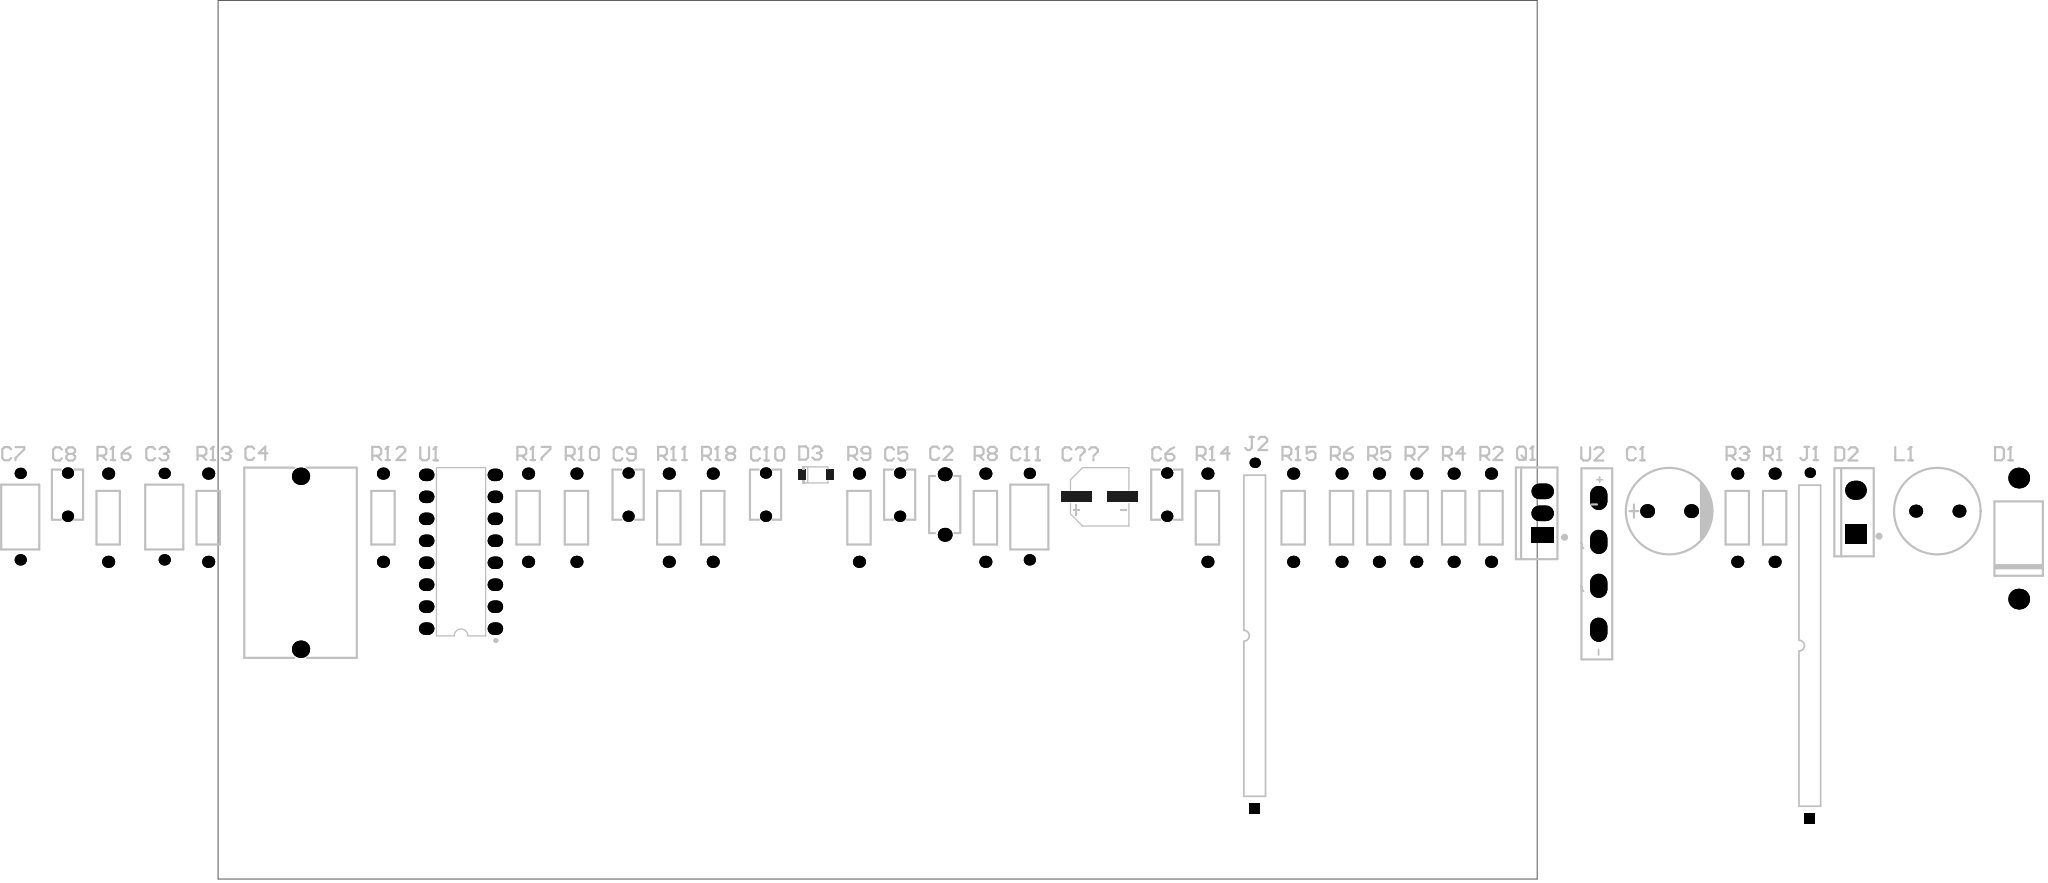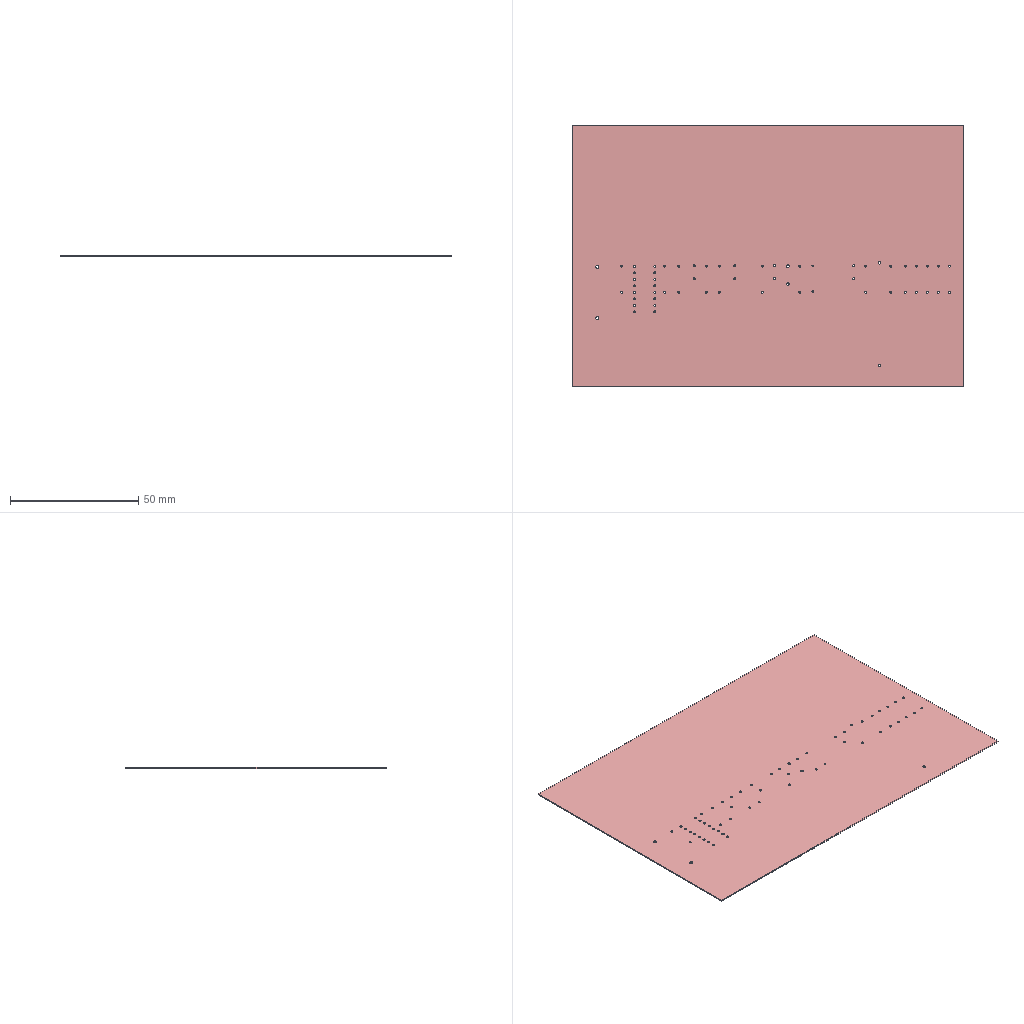Circuit board layout | Altium Designer | box 152.4 x 101.6 x 0.4 mm
Part placement:
Designator,Comment,Layer,Footprint,Center-X(mm),Center-Y(mm),Rotation
U2,GBU8K,TopLayer,GBU_4P-L22.0-W3.5-P5.08-GBU4K,184.912,61.849,90
U1,UC3854N,TopLayer,PDIP-16_L19.3-W6.4-P2.54-LS7.94-BL,53.467,63.246,90
R18,MF1/4W-100K±1%-OT26,TopLayer,RES-TH_BD2.7-L6.2-P10.20-D0.4,82.55,67.183,90
R17,MF1/4W-100K±1%-OT26,TopLayer,RES-TH_BD2.7-L6.2-P10.20-D0.4,61.214,67.183,90
R16,MF1/4W-100K±1%-OT26,TopLayer,RES-TH_BD2.7-L6.2-P10.20-D0.4,12.7,67.183,90
R15,MF1/4W-100K±1%-OT26,TopLayer,RES-TH_BD2.7-L6.2-P10.20-D0.4,149.606,67.183,90
R14,MF1/4W-100K±1%-OT26,TopLayer,RES-TH_BD2.7-L6.2-P10.20-D0.4,139.7,67.183,90
R13,MF1/4W-100K±1%-OT26,TopLayer,RES-TH_BD2.7-L6.2-P10.20-D0.4,24.257,67.183,90
R12,MF1/4W-100K±1%-OT26,TopLayer,RES-TH_BD2.7-L6.2-P10.20-D0.4,44.45,67.183,90
R11,MF1/4W-100K±1%-OT26,TopLayer,RES-TH_BD2.7-L6.2-P10.20-D0.4,77.47,67.183,90
R10,MF1/4W-100K±1%-OT26,TopLayer,RES-TH_BD2.7-L6.2-P10.20-D0.4,66.802,67.183,90
R9,MF1/4W-100K±1%-OT26,TopLayer,RES-TH_BD2.7-L6.2-P10.20-D0.4,99.441,67.183,90
R8,MF1/4W-100K±1%-OT26,TopLayer,RES-TH_BD2.7-L6.2-P10.20-D0.4,114.046,67.183,90
R7,MF1/4W-100K±1%-OT26,TopLayer,RES-TH_BD2.7-L6.2-P10.20-D0.4,163.83,67.183,90
R6,MF1/4W-100K±1%-OT26,TopLayer,RES-TH_BD2.7-L6.2-P10.20-D0.4,155.194,67.183,90
R5,MF1/4W-100K±1%-OT26,TopLayer,RES-TH_BD2.7-L6.2-P10.20-D0.4,159.512,67.183,90
R4,MF1/4W-100K±1%-OT26,TopLayer,RES-TH_BD2.7-L6.2-P10.20-D0.4,168.148,67.183,90
R3,MF1/4W-100K±1%-OT26,TopLayer,RES-TH_BD2.7-L6.2-P10.20-D0.4,200.914,67.183,90
R2,MF1/4W-100K±1%-OT26,TopLayer,RES-TH_BD2.7-L6.2-P10.20-D0.4,172.466,67.183,90
R1,MF1/4W-100K±1%-OT26,TopLayer,RES-TH_BD2.7-L6.2-P10.20-D0.4,205.232,67.183,90
Q1,IRF530NPBF,TopLayer,TO-220-3_L10.0-W4.5-P2.54-L,178.435,67.691,90
L1,XR8*10-101K-L,TopLayer,IND-TH_BD10.0-P5.00-D0.6,224.028,67.945,0
J2,2,TopLayer,DIP2_-_duplicate,145.161,53.533,90
J1,2,TopLayer,DIP2_-_duplicate,209.296,52.385,90
D3,BZT52C8V2_C19077406,TopLayer,SOD-123_L2.7-W1.6-LS3.7-RD,94.488,72.136,0
D2,GC3D10060A,TopLayer,TO-220-2_L10.2-W4.5-P5.08-L-A,214.63,67.818,90
D1,1N5406_C5338388,TopLayer,DO-27_BD5.2-L8.9-P12.90-D1.5-RD,233.426,64.77,90
C??,RVE100UF35V67RV0072,TopLayer,CAP-SMD_BD6.3-L6.6-W6.6-LS7.6-FD-1,127.254,69.596,0
C11,KY1102M400VAC70Y10093,TopLayer,CAP-TH_L7.5-W4.5-P10.00-D0.6,119.126,67.31,90
C10,178MU0002,TopLayer,CAP-TH_L5.8-W3.6-P5.0-D0.6,88.646,69.85,90
C9,178MU0002,TopLayer,CAP-TH_L5.8-W3.6-P5.0-D0.6,72.771,69.85,90
C8,178MU0002,TopLayer,CAP-TH_L5.8-W3.6-P5.0-D0.6,8.001,69.85,90
C7,KY1102M400VAC70Y10093,TopLayer,CAP-TH_L7.5-W4.5-P10.00-D0.6,2.54,67.31,90
C6,178MU0002,TopLayer,CAP-TH_L5.8-W3.6-P5.0-D0.6,135.001,69.85,90
C5,178MU0002,TopLayer,CAP-TH_L5.8-W3.6-P5.0-D0.6,104.14,69.85,90
C4,CBB21-400V/255JP20,TopLayer,CAP-TH_L22.0-W12.5-P20.00-D0.7-FD,34.925,61.976,90
C3,KY1102M400VAC70Y10093,TopLayer,CAP-TH_L7.5-W4.5-P10.00-D0.6,19.177,67.31,90
C2,KJKF222M2FF7035A075E,TopLayer,CAP-TH_L6.5-W3.5-P7.50-D1.0,109.347,68.707,90
C1,LKME1402A101MF,TopLayer,CAP-TH_BD10.0-P5.00-D1.0-FD,193.04,67.945,0